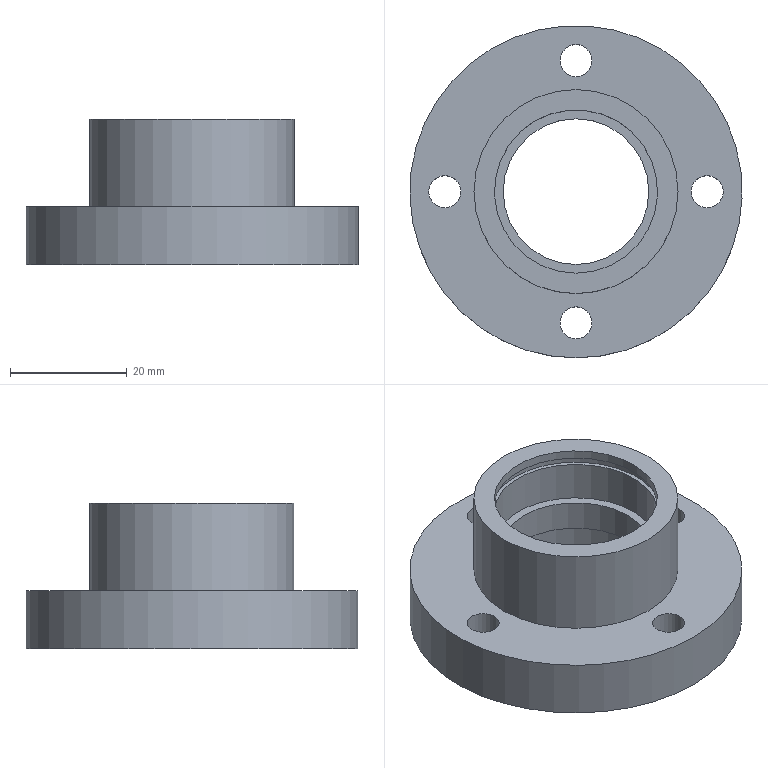Part | NX | features Housing_5003_005_BGRB6902ZZ-25 2 | 1 solid | 30 faces | box 57 x 57 x 25 mm | volume 23135 mm3 | cylinder 17 | plane 13 | commonest cylinder face diameters 5.5 x4 9.5 x4 28 x4 29.4 x2 25 x1 35 x1
STEP:
#1=CARTESIAN_POINT('',(158.525,-336.7,-236.5));
#2=VERTEX_POINT('',#1);
#3=CARTESIAN_POINT('',(158.525,-322.,-236.5));
#4=DIRECTION('',(0.,0.,-1.));
#5=DIRECTION('',(0.,-1.,0.));
#6=AXIS2_PLACEMENT_3D('',#3,#4,#5);
#7=CIRCLE('',#6,14.7);
#8=EDGE_CURVE('',#2,#2,#7,.T.);
#9=ORIENTED_EDGE('',*,*,#8,.T.);
#10=EDGE_LOOP('',(#9));
#11=FACE_BOUND('',#10,.T.);
#12=CARTESIAN_POINT('',(158.525,-336.,-236.5));
#13=VERTEX_POINT('',#12);
#14=CARTESIAN_POINT('',(158.525,-322.,-236.5));
#15=DIRECTION('',(0.,0.,-1.));
#16=DIRECTION('',(0.,-1.,0.));
#17=AXIS2_PLACEMENT_3D('',#14,#15,#16);
#18=CIRCLE('',#17,14.);
#19=EDGE_CURVE('',#13,#13,#18,.T.);
#20=ORIENTED_EDGE('',*,*,#19,.F.);
#21=EDGE_LOOP('',(#20));
#22=FACE_BOUND('',#21,.T.);
#23=CARTESIAN_POINT('',(144.525,-322.,-236.5));
#24=DIRECTION('',(0.,0.,-1.));
#25=DIRECTION('',(0.,-1.,0.));
#26=AXIS2_PLACEMENT_3D('',#23,#24,#25);
#27=PLANE('',#26);
#28=ADVANCED_FACE('',(#11,#22),#27,.T.);
#29=ORIENTED_EDGE('',*,*,#19,.T.);
#30=EDGE_LOOP('',(#29));
#31=FACE_BOUND('',#30,.T.);
#32=CARTESIAN_POINT('',(158.525,-336.,-235.));
#33=VERTEX_POINT('',#32);
#34=CARTESIAN_POINT('',(158.525,-322.,-235.));
#35=DIRECTION('',(0.,0.,-1.));
#36=DIRECTION('',(0.,-1.,0.));
#37=AXIS2_PLACEMENT_3D('',#34,#35,#36);
#38=CIRCLE('',#37,14.);
#39=EDGE_CURVE('',#33,#33,#38,.T.);
#40=ORIENTED_EDGE('',*,*,#39,.F.);
#41=EDGE_LOOP('',(#40));
#42=FACE_BOUND('',#41,.T.);
#43=CARTESIAN_POINT('',(158.525,-322.,-260.));
#44=DIRECTION('',(0.,0.,-1.));
#45=DIRECTION('',(0.,-1.,0.));
#46=AXIS2_PLACEMENT_3D('',#43,#44,#45);
#47=CYLINDRICAL_SURFACE('',#46,14.);
#48=ADVANCED_FACE('',(#31,#42),#47,.F.);
#49=ORIENTED_EDGE('',*,*,#39,.T.);
#50=EDGE_LOOP('',(#49));
#51=FACE_BOUND('',#50,.T.);
#52=CARTESIAN_POINT('',(158.525,-339.5,-235.));
#53=VERTEX_POINT('',#52);
#54=CARTESIAN_POINT('',(158.525,-322.,-235.));
#55=DIRECTION('',(0.,0.,-1.));
#56=DIRECTION('',(0.,-1.,0.));
#57=AXIS2_PLACEMENT_3D('',#54,#55,#56);
#58=CIRCLE('',#57,17.5);
#59=EDGE_CURVE('',#53,#53,#58,.T.);
#60=ORIENTED_EDGE('',*,*,#59,.F.);
#61=EDGE_LOOP('',(#60));
#62=FACE_BOUND('',#61,.T.);
#63=CARTESIAN_POINT('',(141.025,-322.,-235.));
#64=DIRECTION('',(0.,0.,1.));
#65=DIRECTION('',(0.,1.,0.));
#66=AXIS2_PLACEMENT_3D('',#63,#64,#65);
#67=PLANE('',#66);
#68=ADVANCED_FACE('',(#51,#62),#67,.T.);
#69=ORIENTED_EDGE('',*,*,#59,.T.);
#70=EDGE_LOOP('',(#69));
#71=FACE_BOUND('',#70,.T.);
#72=CARTESIAN_POINT('',(158.525,-339.5,-250.));
#73=VERTEX_POINT('',#72);
#74=CARTESIAN_POINT('',(158.525,-322.,-250.));
#75=DIRECTION('',(0.,0.,-1.));
#76=DIRECTION('',(0.,-1.,0.));
#77=AXIS2_PLACEMENT_3D('',#74,#75,#76);
#78=CIRCLE('',#77,17.5);
#79=EDGE_CURVE('',#73,#73,#78,.T.);
#80=ORIENTED_EDGE('',*,*,#79,.F.);
#81=EDGE_LOOP('',(#80));
#82=FACE_BOUND('',#81,.T.);
#83=CARTESIAN_POINT('',(158.525,-322.,-260.));
#84=DIRECTION('',(0.,0.,-1.));
#85=DIRECTION('',(0.,-1.,0.));
#86=AXIS2_PLACEMENT_3D('',#83,#84,#85);
#87=CYLINDRICAL_SURFACE('',#86,17.5);
#88=ADVANCED_FACE('',(#71,#82),#87,.T.);
#89=CARTESIAN_POINT('',(136.025,-319.25,-250.));
#90=VERTEX_POINT('',#89);
#91=CARTESIAN_POINT('',(136.025,-322.,-250.));
#92=DIRECTION('',(0.,0.,1.));
#93=DIRECTION('',(0.,1.,0.));
#94=AXIS2_PLACEMENT_3D('',#91,#92,#93);
#95=CIRCLE('',#94,2.75);
#96=EDGE_CURVE('',#90,#90,#95,.T.);
#97=ORIENTED_EDGE('',*,*,#96,.F.);
#98=EDGE_LOOP('',(#97));
#99=FACE_BOUND('',#98,.T.);
#100=CARTESIAN_POINT('',(158.525,-341.75,-250.));
#101=VERTEX_POINT('',#100);
#102=CARTESIAN_POINT('',(158.525,-344.5,-250.));
#103=DIRECTION('',(0.,0.,1.));
#104=DIRECTION('',(0.,1.,0.));
#105=AXIS2_PLACEMENT_3D('',#102,#103,#104);
#106=CIRCLE('',#105,2.75);
#107=EDGE_CURVE('',#101,#101,#106,.T.);
#108=ORIENTED_EDGE('',*,*,#107,.F.);
#109=EDGE_LOOP('',(#108));
#110=FACE_BOUND('',#109,.T.);
#111=CARTESIAN_POINT('',(158.525,-296.75,-250.));
#112=VERTEX_POINT('',#111);
#113=CARTESIAN_POINT('',(158.525,-299.5,-250.));
#114=DIRECTION('',(0.,0.,1.));
#115=DIRECTION('',(0.,1.,0.));
#116=AXIS2_PLACEMENT_3D('',#113,#114,#115);
#117=CIRCLE('',#116,2.75);
#118=EDGE_CURVE('',#112,#112,#117,.T.);
#119=ORIENTED_EDGE('',*,*,#118,.F.);
#120=EDGE_LOOP('',(#119));
#121=FACE_BOUND('',#120,.T.);
#122=CARTESIAN_POINT('',(181.025,-319.25,-250.));
#123=VERTEX_POINT('',#122);
#124=CARTESIAN_POINT('',(181.025,-322.,-250.));
#125=DIRECTION('',(0.,0.,1.));
#126=DIRECTION('',(0.,1.,0.));
#127=AXIS2_PLACEMENT_3D('',#124,#125,#126);
#128=CIRCLE('',#127,2.75);
#129=EDGE_CURVE('',#123,#123,#128,.T.);
#130=ORIENTED_EDGE('',*,*,#129,.F.);
#131=EDGE_LOOP('',(#130));
#132=FACE_BOUND('',#131,.T.);
#133=ORIENTED_EDGE('',*,*,#79,.T.);
#134=EDGE_LOOP('',(#133));
#135=FACE_BOUND('',#134,.T.);
#136=CARTESIAN_POINT('',(158.525,-350.5,-250.));
#137=VERTEX_POINT('',#136);
#138=CARTESIAN_POINT('',(158.525,-322.,-250.));
#139=DIRECTION('',(0.,0.,-1.));
#140=DIRECTION('',(0.,-1.,0.));
#141=AXIS2_PLACEMENT_3D('',#138,#139,#140);
#142=CIRCLE('',#141,28.5);
#143=EDGE_CURVE('',#137,#137,#142,.T.);
#144=ORIENTED_EDGE('',*,*,#143,.F.);
#145=EDGE_LOOP('',(#144));
#146=FACE_BOUND('',#145,.T.);
#147=CARTESIAN_POINT('',(130.025,-322.,-250.));
#148=DIRECTION('',(0.,0.,1.));
#149=DIRECTION('',(0.,1.,0.));
#150=AXIS2_PLACEMENT_3D('',#147,#148,#149);
#151=PLANE('',#150);
#152=ADVANCED_FACE('',(#99,#110,#121,#132,#135,#146),#151,.T.);
#153=ORIENTED_EDGE('',*,*,#143,.T.);
#154=EDGE_LOOP('',(#153));
#155=FACE_BOUND('',#154,.T.);
#156=CARTESIAN_POINT('',(158.525,-350.5,-260.));
#157=VERTEX_POINT('',#156);
#158=CARTESIAN_POINT('',(158.525,-322.,-260.));
#159=DIRECTION('',(0.,0.,-1.));
#160=DIRECTION('',(0.,-1.,0.));
#161=AXIS2_PLACEMENT_3D('',#158,#159,#160);
#162=CIRCLE('',#161,28.5);
#163=EDGE_CURVE('',#157,#157,#162,.T.);
#164=ORIENTED_EDGE('',*,*,#163,.F.);
#165=EDGE_LOOP('',(#164));
#166=FACE_BOUND('',#165,.T.);
#167=CARTESIAN_POINT('',(158.525,-322.,-260.));
#168=DIRECTION('',(0.,0.,-1.));
#169=DIRECTION('',(0.,-1.,0.));
#170=AXIS2_PLACEMENT_3D('',#167,#168,#169);
#171=CYLINDRICAL_SURFACE('',#170,28.5);
#172=ADVANCED_FACE('',(#155,#166),#171,.T.);
#173=CARTESIAN_POINT('',(136.025,-326.75,-260.));
#174=VERTEX_POINT('',#173);
#175=CARTESIAN_POINT('',(136.025,-322.,-260.));
#176=DIRECTION('',(0.,0.,-1.));
#177=DIRECTION('',(0.,-1.,0.));
#178=AXIS2_PLACEMENT_3D('',#175,#176,#177);
#179=CIRCLE('',#178,4.75);
#180=EDGE_CURVE('',#174,#174,#179,.T.);
#181=ORIENTED_EDGE('',*,*,#180,.F.);
#182=EDGE_LOOP('',(#181));
#183=FACE_BOUND('',#182,.T.);
#184=CARTESIAN_POINT('',(158.525,-349.25,-260.));
#185=VERTEX_POINT('',#184);
#186=CARTESIAN_POINT('',(158.525,-344.5,-260.));
#187=DIRECTION('',(0.,0.,-1.));
#188=DIRECTION('',(0.,-1.,0.));
#189=AXIS2_PLACEMENT_3D('',#186,#187,#188);
#190=CIRCLE('',#189,4.75);
#191=EDGE_CURVE('',#185,#185,#190,.T.);
#192=ORIENTED_EDGE('',*,*,#191,.F.);
#193=EDGE_LOOP('',(#192));
#194=FACE_BOUND('',#193,.T.);
#195=CARTESIAN_POINT('',(158.525,-304.25,-260.));
#196=VERTEX_POINT('',#195);
#197=CARTESIAN_POINT('',(158.525,-299.5,-260.));
#198=DIRECTION('',(0.,0.,-1.));
#199=DIRECTION('',(0.,-1.,0.));
#200=AXIS2_PLACEMENT_3D('',#197,#198,#199);
#201=CIRCLE('',#200,4.75);
#202=EDGE_CURVE('',#196,#196,#201,.T.);
#203=ORIENTED_EDGE('',*,*,#202,.F.);
#204=EDGE_LOOP('',(#203));
#205=FACE_BOUND('',#204,.T.);
#206=CARTESIAN_POINT('',(181.025,-326.75,-260.));
#207=VERTEX_POINT('',#206);
#208=CARTESIAN_POINT('',(181.025,-322.,-260.));
#209=DIRECTION('',(0.,0.,-1.));
#210=DIRECTION('',(0.,-1.,0.));
#211=AXIS2_PLACEMENT_3D('',#208,#209,#210);
#212=CIRCLE('',#211,4.75);
#213=EDGE_CURVE('',#207,#207,#212,.T.);
#214=ORIENTED_EDGE('',*,*,#213,.F.);
#215=EDGE_LOOP('',(#214));
#216=FACE_BOUND('',#215,.T.);
#217=ORIENTED_EDGE('',*,*,#163,.T.);
#218=EDGE_LOOP('',(#217));
#219=FACE_BOUND('',#218,.T.);
#220=CARTESIAN_POINT('',(158.525,-336.,-260.));
#221=VERTEX_POINT('',#220);
#222=CARTESIAN_POINT('',(158.525,-322.,-260.));
#223=DIRECTION('',(0.,0.,-1.));
#224=DIRECTION('',(0.,-1.,0.));
#225=AXIS2_PLACEMENT_3D('',#222,#223,#224);
#226=CIRCLE('',#225,14.);
#227=EDGE_CURVE('',#221,#221,#226,.T.);
#228=ORIENTED_EDGE('',*,*,#227,.F.);
#229=EDGE_LOOP('',(#228));
#230=FACE_BOUND('',#229,.T.);
#231=CARTESIAN_POINT('',(144.525,-322.,-260.));
#232=DIRECTION('',(0.,0.,-1.));
#233=DIRECTION('',(0.,-1.,0.));
#234=AXIS2_PLACEMENT_3D('',#231,#232,#233);
#235=PLANE('',#234);
#236=ADVANCED_FACE('',(#183,#194,#205,#216,#219,#230),#235,.T.);
#237=ORIENTED_EDGE('',*,*,#227,.T.);
#238=EDGE_LOOP('',(#237));
#239=FACE_BOUND('',#238,.T.);
#240=CARTESIAN_POINT('',(158.525,-336.,-258.5));
#241=VERTEX_POINT('',#240);
#242=CARTESIAN_POINT('',(158.525,-322.,-258.5));
#243=DIRECTION('',(0.,0.,-1.));
#244=DIRECTION('',(0.,-1.,0.));
#245=AXIS2_PLACEMENT_3D('',#242,#243,#244);
#246=CIRCLE('',#245,14.);
#247=EDGE_CURVE('',#241,#241,#246,.T.);
#248=ORIENTED_EDGE('',*,*,#247,.F.);
#249=EDGE_LOOP('',(#248));
#250=FACE_BOUND('',#249,.T.);
#251=CARTESIAN_POINT('',(158.525,-322.,-260.));
#252=DIRECTION('',(0.,0.,-1.));
#253=DIRECTION('',(0.,-1.,0.));
#254=AXIS2_PLACEMENT_3D('',#251,#252,#253);
#255=CYLINDRICAL_SURFACE('',#254,14.);
#256=ADVANCED_FACE('',(#239,#250),#255,.F.);
#257=ORIENTED_EDGE('',*,*,#247,.T.);
#258=EDGE_LOOP('',(#257));
#259=FACE_BOUND('',#258,.T.);
#260=CARTESIAN_POINT('',(158.525,-336.7,-258.5));
#261=VERTEX_POINT('',#260);
#262=CARTESIAN_POINT('',(158.525,-322.,-258.5));
#263=DIRECTION('',(0.,0.,-1.));
#264=DIRECTION('',(0.,-1.,0.));
#265=AXIS2_PLACEMENT_3D('',#262,#263,#264);
#266=CIRCLE('',#265,14.7);
#267=EDGE_CURVE('',#261,#261,#266,.T.);
#268=ORIENTED_EDGE('',*,*,#267,.F.);
#269=EDGE_LOOP('',(#268));
#270=FACE_BOUND('',#269,.T.);
#271=CARTESIAN_POINT('',(143.825,-322.,-258.5));
#272=DIRECTION('',(0.,0.,1.));
#273=DIRECTION('',(0.,1.,0.));
#274=AXIS2_PLACEMENT_3D('',#271,#272,#273);
#275=PLANE('',#274);
#276=ADVANCED_FACE('',(#259,#270),#275,.T.);
#277=ORIENTED_EDGE('',*,*,#267,.T.);
#278=EDGE_LOOP('',(#277));
#279=FACE_BOUND('',#278,.T.);
#280=CARTESIAN_POINT('',(158.525,-336.7,-257.15));
#281=VERTEX_POINT('',#280);
#282=CARTESIAN_POINT('',(158.525,-322.,-257.15));
#283=DIRECTION('',(0.,0.,-1.));
#284=DIRECTION('',(0.,-1.,0.));
#285=AXIS2_PLACEMENT_3D('',#282,#283,#284);
#286=CIRCLE('',#285,14.7);
#287=EDGE_CURVE('',#281,#281,#286,.T.);
#288=ORIENTED_EDGE('',*,*,#287,.F.);
#289=EDGE_LOOP('',(#288));
#290=FACE_BOUND('',#289,.T.);
#291=CARTESIAN_POINT('',(158.525,-322.,-260.));
#292=DIRECTION('',(0.,0.,-1.));
#293=DIRECTION('',(0.,-1.,0.));
#294=AXIS2_PLACEMENT_3D('',#291,#292,#293);
#295=CYLINDRICAL_SURFACE('',#294,14.7);
#296=ADVANCED_FACE('',(#279,#290),#295,.F.);
#297=ORIENTED_EDGE('',*,*,#287,.T.);
#298=EDGE_LOOP('',(#297));
#299=FACE_BOUND('',#298,.T.);
#300=CARTESIAN_POINT('',(158.525,-336.,-257.15));
#301=VERTEX_POINT('',#300);
#302=CARTESIAN_POINT('',(158.525,-322.,-257.15));
#303=DIRECTION('',(0.,0.,-1.));
#304=DIRECTION('',(0.,-1.,0.));
#305=AXIS2_PLACEMENT_3D('',#302,#303,#304);
#306=CIRCLE('',#305,14.);
#307=EDGE_CURVE('',#301,#301,#306,.T.);
#308=ORIENTED_EDGE('',*,*,#307,.F.);
#309=EDGE_LOOP('',(#308));
#310=FACE_BOUND('',#309,.T.);
#311=CARTESIAN_POINT('',(144.525,-322.,-257.15));
#312=DIRECTION('',(0.,0.,-1.));
#313=DIRECTION('',(0.,-1.,0.));
#314=AXIS2_PLACEMENT_3D('',#311,#312,#313);
#315=PLANE('',#314);
#316=ADVANCED_FACE('',(#299,#310),#315,.T.);
#317=ORIENTED_EDGE('',*,*,#307,.T.);
#318=EDGE_LOOP('',(#317));
#319=FACE_BOUND('',#318,.T.);
#320=CARTESIAN_POINT('',(158.525,-336.,-250.15));
#321=VERTEX_POINT('',#320);
#322=CARTESIAN_POINT('',(158.525,-322.,-250.15));
#323=DIRECTION('',(0.,0.,-1.));
#324=DIRECTION('',(0.,-1.,0.));
#325=AXIS2_PLACEMENT_3D('',#322,#323,#324);
#326=CIRCLE('',#325,14.);
#327=EDGE_CURVE('',#321,#321,#326,.T.);
#328=ORIENTED_EDGE('',*,*,#327,.F.);
#329=EDGE_LOOP('',(#328));
#330=FACE_BOUND('',#329,.T.);
#331=CARTESIAN_POINT('',(158.525,-322.,-260.));
#332=DIRECTION('',(0.,0.,-1.));
#333=DIRECTION('',(0.,-1.,0.));
#334=AXIS2_PLACEMENT_3D('',#331,#332,#333);
#335=CYLINDRICAL_SURFACE('',#334,14.);
#336=ADVANCED_FACE('',(#319,#330),#335,.F.);
#337=ORIENTED_EDGE('',*,*,#327,.T.);
#338=EDGE_LOOP('',(#337));
#339=FACE_BOUND('',#338,.T.);
#340=CARTESIAN_POINT('',(158.525,-334.5,-250.15));
#341=VERTEX_POINT('',#340);
#342=CARTESIAN_POINT('',(158.525,-322.,-250.15));
#343=DIRECTION('',(0.,0.,-1.));
#344=DIRECTION('',(0.,-1.,0.));
#345=AXIS2_PLACEMENT_3D('',#342,#343,#344);
#346=CIRCLE('',#345,12.5);
#347=EDGE_CURVE('',#341,#341,#346,.T.);
#348=ORIENTED_EDGE('',*,*,#347,.F.);
#349=EDGE_LOOP('',(#348));
#350=FACE_BOUND('',#349,.T.);
#351=CARTESIAN_POINT('',(146.025,-322.,-250.15));
#352=DIRECTION('',(0.,0.,-1.));
#353=DIRECTION('',(0.,-1.,0.));
#354=AXIS2_PLACEMENT_3D('',#351,#352,#353);
#355=PLANE('',#354);
#356=ADVANCED_FACE('',(#339,#350),#355,.T.);
#357=ORIENTED_EDGE('',*,*,#347,.T.);
#358=EDGE_LOOP('',(#357));
#359=FACE_BOUND('',#358,.T.);
#360=CARTESIAN_POINT('',(158.525,-334.5,-244.85));
#361=VERTEX_POINT('',#360);
#362=CARTESIAN_POINT('',(158.525,-322.,-244.85));
#363=DIRECTION('',(0.,0.,-1.));
#364=DIRECTION('',(0.,-1.,0.));
#365=AXIS2_PLACEMENT_3D('',#362,#363,#364);
#366=CIRCLE('',#365,12.5);
#367=EDGE_CURVE('',#361,#361,#366,.T.);
#368=ORIENTED_EDGE('',*,*,#367,.F.);
#369=EDGE_LOOP('',(#368));
#370=FACE_BOUND('',#369,.T.);
#371=CARTESIAN_POINT('',(158.525,-322.,-260.));
#372=DIRECTION('',(0.,0.,-1.));
#373=DIRECTION('',(0.,-1.,0.));
#374=AXIS2_PLACEMENT_3D('',#371,#372,#373);
#375=CYLINDRICAL_SURFACE('',#374,12.5);
#376=ADVANCED_FACE('',(#359,#370),#375,.F.);
#377=ORIENTED_EDGE('',*,*,#367,.T.);
#378=EDGE_LOOP('',(#377));
#379=FACE_BOUND('',#378,.T.);
#380=CARTESIAN_POINT('',(158.525,-336.,-244.85));
#381=VERTEX_POINT('',#380);
#382=CARTESIAN_POINT('',(158.525,-322.,-244.85));
#383=DIRECTION('',(0.,0.,-1.));
#384=DIRECTION('',(0.,-1.,0.));
#385=AXIS2_PLACEMENT_3D('',#382,#383,#384);
#386=CIRCLE('',#385,14.);
#387=EDGE_CURVE('',#381,#381,#386,.T.);
#388=ORIENTED_EDGE('',*,*,#387,.F.);
#389=EDGE_LOOP('',(#388));
#390=FACE_BOUND('',#389,.T.);
#391=CARTESIAN_POINT('',(144.525,-322.,-244.85));
#392=DIRECTION('',(0.,0.,1.));
#393=DIRECTION('',(0.,1.,0.));
#394=AXIS2_PLACEMENT_3D('',#391,#392,#393);
#395=PLANE('',#394);
#396=ADVANCED_FACE('',(#379,#390),#395,.T.);
#397=ORIENTED_EDGE('',*,*,#387,.T.);
#398=EDGE_LOOP('',(#397));
#399=FACE_BOUND('',#398,.T.);
#400=CARTESIAN_POINT('',(158.525,-336.,-237.85));
#401=VERTEX_POINT('',#400);
#402=CARTESIAN_POINT('',(158.525,-322.,-237.85));
#403=DIRECTION('',(0.,0.,-1.));
#404=DIRECTION('',(0.,-1.,0.));
#405=AXIS2_PLACEMENT_3D('',#402,#403,#404);
#406=CIRCLE('',#405,14.);
#407=EDGE_CURVE('',#401,#401,#406,.T.);
#408=ORIENTED_EDGE('',*,*,#407,.F.);
#409=EDGE_LOOP('',(#408));
#410=FACE_BOUND('',#409,.T.);
#411=CARTESIAN_POINT('',(158.525,-322.,-260.));
#412=DIRECTION('',(0.,0.,-1.));
#413=DIRECTION('',(0.,-1.,0.));
#414=AXIS2_PLACEMENT_3D('',#411,#412,#413);
#415=CYLINDRICAL_SURFACE('',#414,14.);
#416=ADVANCED_FACE('',(#399,#410),#415,.F.);
#417=ORIENTED_EDGE('',*,*,#407,.T.);
#418=EDGE_LOOP('',(#417));
#419=FACE_BOUND('',#418,.T.);
#420=CARTESIAN_POINT('',(158.525,-336.7,-237.85));
#421=VERTEX_POINT('',#420);
#422=CARTESIAN_POINT('',(158.525,-322.,-237.85));
#423=DIRECTION('',(0.,0.,-1.));
#424=DIRECTION('',(0.,-1.,0.));
#425=AXIS2_PLACEMENT_3D('',#422,#423,#424);
#426=CIRCLE('',#425,14.7);
#427=EDGE_CURVE('',#421,#421,#426,.T.);
#428=ORIENTED_EDGE('',*,*,#427,.F.);
#429=EDGE_LOOP('',(#428));
#430=FACE_BOUND('',#429,.T.);
#431=CARTESIAN_POINT('',(143.825,-322.,-237.85));
#432=DIRECTION('',(0.,0.,1.));
#433=DIRECTION('',(0.,1.,0.));
#434=AXIS2_PLACEMENT_3D('',#431,#432,#433);
#435=PLANE('',#434);
#436=ADVANCED_FACE('',(#419,#430),#435,.T.);
#437=ORIENTED_EDGE('',*,*,#427,.T.);
#438=EDGE_LOOP('',(#437));
#439=FACE_BOUND('',#438,.T.);
#440=ORIENTED_EDGE('',*,*,#8,.F.);
#441=EDGE_LOOP('',(#440));
#442=FACE_BOUND('',#441,.T.);
#443=CARTESIAN_POINT('',(158.525,-322.,-260.));
#444=DIRECTION('',(0.,0.,-1.));
#445=DIRECTION('',(0.,-1.,0.));
#446=AXIS2_PLACEMENT_3D('',#443,#444,#445);
#447=CYLINDRICAL_SURFACE('',#446,14.7);
#448=ADVANCED_FACE('',(#439,#442),#447,.F.);
#449=ORIENTED_EDGE('',*,*,#129,.T.);
#450=EDGE_LOOP('',(#449));
#451=FACE_BOUND('',#450,.T.);
#452=CARTESIAN_POINT('',(181.025,-324.75,-254.9));
#453=VERTEX_POINT('',#452);
#454=CARTESIAN_POINT('',(181.025,-322.,-254.9));
#455=DIRECTION('',(0.,0.,-1.));
#456=DIRECTION('',(0.,-1.,0.));
#457=AXIS2_PLACEMENT_3D('',#454,#455,#456);
#458=CIRCLE('',#457,2.75);
#459=EDGE_CURVE('',#453,#453,#458,.T.);
#460=ORIENTED_EDGE('',*,*,#459,.T.);
#461=EDGE_LOOP('',(#460));
#462=FACE_BOUND('',#461,.T.);
#463=CARTESIAN_POINT('',(181.025,-322.,-260.));
#464=DIRECTION('',(0.,0.,-1.));
#465=DIRECTION('',(0.,-1.,0.));
#466=AXIS2_PLACEMENT_3D('',#463,#464,#465);
#467=CYLINDRICAL_SURFACE('',#466,2.75);
#468=ADVANCED_FACE('',(#451,#462),#467,.F.);
#469=ORIENTED_EDGE('',*,*,#459,.F.);
#470=EDGE_LOOP('',(#469));
#471=FACE_BOUND('',#470,.T.);
#472=CARTESIAN_POINT('',(181.025,-326.75,-254.9));
#473=VERTEX_POINT('',#472);
#474=CARTESIAN_POINT('',(181.025,-322.,-254.9));
#475=DIRECTION('',(0.,0.,-1.));
#476=DIRECTION('',(0.,-1.,0.));
#477=AXIS2_PLACEMENT_3D('',#474,#475,#476);
#478=CIRCLE('',#477,4.75);
#479=EDGE_CURVE('',#473,#473,#478,.T.);
#480=ORIENTED_EDGE('',*,*,#479,.T.);
#481=EDGE_LOOP('',(#480));
#482=FACE_BOUND('',#481,.T.);
#483=CARTESIAN_POINT('',(178.275,-322.,-254.9));
#484=DIRECTION('',(0.,0.,1.));
#485=DIRECTION('',(0.,1.,0.));
#486=AXIS2_PLACEMENT_3D('',#483,#484,#485);
#487=PLANE('',#486);
#488=ADVANCED_FACE('',(#471,#482),#487,.F.);
#489=ORIENTED_EDGE('',*,*,#479,.F.);
#490=EDGE_LOOP('',(#489));
#491=FACE_BOUND('',#490,.T.);
#492=ORIENTED_EDGE('',*,*,#213,.T.);
#493=EDGE_LOOP('',(#492));
#494=FACE_BOUND('',#493,.T.);
#495=CARTESIAN_POINT('',(181.025,-322.,-260.));
#496=DIRECTION('',(0.,0.,-1.));
#497=DIRECTION('',(0.,-1.,0.));
#498=AXIS2_PLACEMENT_3D('',#495,#496,#497);
#499=CYLINDRICAL_SURFACE('',#498,4.75);
#500=ADVANCED_FACE('',(#491,#494),#499,.F.);
#501=ORIENTED_EDGE('',*,*,#118,.T.);
#502=EDGE_LOOP('',(#501));
#503=FACE_BOUND('',#502,.T.);
#504=CARTESIAN_POINT('',(158.525,-302.25,-254.9));
#505=VERTEX_POINT('',#504);
#506=CARTESIAN_POINT('',(158.525,-299.5,-254.9));
#507=DIRECTION('',(0.,0.,-1.));
#508=DIRECTION('',(0.,-1.,0.));
#509=AXIS2_PLACEMENT_3D('',#506,#507,#508);
#510=CIRCLE('',#509,2.75);
#511=EDGE_CURVE('',#505,#505,#510,.T.);
#512=ORIENTED_EDGE('',*,*,#511,.T.);
#513=EDGE_LOOP('',(#512));
#514=FACE_BOUND('',#513,.T.);
#515=CARTESIAN_POINT('',(158.525,-299.5,-260.));
#516=DIRECTION('',(0.,0.,-1.));
#517=DIRECTION('',(0.,-1.,0.));
#518=AXIS2_PLACEMENT_3D('',#515,#516,#517);
#519=CYLINDRICAL_SURFACE('',#518,2.75);
#520=ADVANCED_FACE('',(#503,#514),#519,.F.);
#521=ORIENTED_EDGE('',*,*,#511,.F.);
#522=EDGE_LOOP('',(#521));
#523=FACE_BOUND('',#522,.T.);
#524=CARTESIAN_POINT('',(158.525,-304.25,-254.9));
#525=VERTEX_POINT('',#524);
#526=CARTESIAN_POINT('',(158.525,-299.5,-254.9));
#527=DIRECTION('',(0.,0.,-1.));
#528=DIRECTION('',(0.,-1.,0.));
#529=AXIS2_PLACEMENT_3D('',#526,#527,#528);
#530=CIRCLE('',#529,4.75);
#531=EDGE_CURVE('',#525,#525,#530,.T.);
#532=ORIENTED_EDGE('',*,*,#531,.T.);
#533=EDGE_LOOP('',(#532));
#534=FACE_BOUND('',#533,.T.);
#535=CARTESIAN_POINT('',(155.775,-299.5,-254.9));
#536=DIRECTION('',(0.,0.,1.));
#537=DIRECTION('',(0.,1.,0.));
#538=AXIS2_PLACEMENT_3D('',#535,#536,#537);
#539=PLANE('',#538);
#540=ADVANCED_FACE('',(#523,#534),#539,.F.);
#541=ORIENTED_EDGE('',*,*,#531,.F.);
#542=EDGE_LOOP('',(#541));
#543=FACE_BOUND('',#542,.T.);
#544=ORIENTED_EDGE('',*,*,#202,.T.);
#545=EDGE_LOOP('',(#544));
#546=FACE_BOUND('',#545,.T.);
#547=CARTESIAN_POINT('',(158.525,-299.5,-260.));
#548=DIRECTION('',(0.,0.,-1.));
#549=DIRECTION('',(0.,-1.,0.));
#550=AXIS2_PLACEMENT_3D('',#547,#548,#549);
#551=CYLINDRICAL_SURFACE('',#550,4.75);
#552=ADVANCED_FACE('',(#543,#546),#551,.F.);
#553=ORIENTED_EDGE('',*,*,#107,.T.);
#554=EDGE_LOOP('',(#553));
#555=FACE_BOUND('',#554,.T.);
#556=CARTESIAN_POINT('',(158.525,-347.25,-254.9));
#557=VERTEX_POINT('',#556);
#558=CARTESIAN_POINT('',(158.525,-344.5,-254.9));
#559=DIRECTION('',(0.,0.,-1.));
#560=DIRECTION('',(0.,-1.,0.));
#561=AXIS2_PLACEMENT_3D('',#558,#559,#560);
#562=CIRCLE('',#561,2.75);
#563=EDGE_CURVE('',#557,#557,#562,.T.);
#564=ORIENTED_EDGE('',*,*,#563,.T.);
#565=EDGE_LOOP('',(#564));
#566=FACE_BOUND('',#565,.T.);
#567=CARTESIAN_POINT('',(158.525,-344.5,-260.));
#568=DIRECTION('',(0.,0.,-1.));
#569=DIRECTION('',(0.,-1.,0.));
#570=AXIS2_PLACEMENT_3D('',#567,#568,#569);
#571=CYLINDRICAL_SURFACE('',#570,2.75);
#572=ADVANCED_FACE('',(#555,#566),#571,.F.);
#573=ORIENTED_EDGE('',*,*,#563,.F.);
#574=EDGE_LOOP('',(#573));
#575=FACE_BOUND('',#574,.T.);
#576=CARTESIAN_POINT('',(158.525,-349.25,-254.9));
#577=VERTEX_POINT('',#576);
#578=CARTESIAN_POINT('',(158.525,-344.5,-254.9));
#579=DIRECTION('',(0.,0.,-1.));
#580=DIRECTION('',(0.,-1.,0.));
#581=AXIS2_PLACEMENT_3D('',#578,#579,#580);
#582=CIRCLE('',#581,4.75);
#583=EDGE_CURVE('',#577,#577,#582,.T.);
#584=ORIENTED_EDGE('',*,*,#583,.T.);
#585=EDGE_LOOP('',(#584));
#586=FACE_BOUND('',#585,.T.);
#587=CARTESIAN_POINT('',(155.775,-344.5,-254.9));
#588=DIRECTION('',(0.,0.,1.));
#589=DIRECTION('',(0.,1.,0.));
#590=AXIS2_PLACEMENT_3D('',#587,#588,#589);
#591=PLANE('',#590);
#592=ADVANCED_FACE('',(#575,#586),#591,.F.);
#593=ORIENTED_EDGE('',*,*,#583,.F.);
#594=EDGE_LOOP('',(#593));
#595=FACE_BOUND('',#594,.T.);
#596=ORIENTED_EDGE('',*,*,#191,.T.);
#597=EDGE_LOOP('',(#596));
#598=FACE_BOUND('',#597,.T.);
#599=CARTESIAN_POINT('',(158.525,-344.5,-260.));
#600=DIRECTION('',(0.,0.,-1.));
#601=DIRECTION('',(0.,-1.,0.));
#602=AXIS2_PLACEMENT_3D('',#599,#600,#601);
#603=CYLINDRICAL_SURFACE('',#602,4.75);
#604=ADVANCED_FACE('',(#595,#598),#603,.F.);
#605=ORIENTED_EDGE('',*,*,#96,.T.);
#606=EDGE_LOOP('',(#605));
#607=FACE_BOUND('',#606,.T.);
#608=CARTESIAN_POINT('',(136.025,-324.75,-254.9));
#609=VERTEX_POINT('',#608);
#610=CARTESIAN_POINT('',(136.025,-322.,-254.9));
#611=DIRECTION('',(0.,0.,-1.));
#612=DIRECTION('',(0.,-1.,0.));
#613=AXIS2_PLACEMENT_3D('',#610,#611,#612);
#614=CIRCLE('',#613,2.75);
#615=EDGE_CURVE('',#609,#609,#614,.T.);
#616=ORIENTED_EDGE('',*,*,#615,.T.);
#617=EDGE_LOOP('',(#616));
#618=FACE_BOUND('',#617,.T.);
#619=CARTESIAN_POINT('',(136.025,-322.,-260.));
#620=DIRECTION('',(0.,0.,-1.));
#621=DIRECTION('',(0.,-1.,0.));
#622=AXIS2_PLACEMENT_3D('',#619,#620,#621);
#623=CYLINDRICAL_SURFACE('',#622,2.75);
#624=ADVANCED_FACE('',(#607,#618),#623,.F.);
#625=ORIENTED_EDGE('',*,*,#615,.F.);
#626=EDGE_LOOP('',(#625));
#627=FACE_BOUND('',#626,.T.);
#628=CARTESIAN_POINT('',(136.025,-326.75,-254.9));
#629=VERTEX_POINT('',#628);
#630=CARTESIAN_POINT('',(136.025,-322.,-254.9));
#631=DIRECTION('',(0.,0.,-1.));
#632=DIRECTION('',(0.,-1.,0.));
#633=AXIS2_PLACEMENT_3D('',#630,#631,#632);
#634=CIRCLE('',#633,4.75);
#635=EDGE_CURVE('',#629,#629,#634,.T.);
#636=ORIENTED_EDGE('',*,*,#635,.T.);
#637=EDGE_LOOP('',(#636));
#638=FACE_BOUND('',#637,.T.);
#639=CARTESIAN_POINT('',(133.275,-322.,-254.9));
#640=DIRECTION('',(0.,0.,1.));
#641=DIRECTION('',(0.,1.,0.));
#642=AXIS2_PLACEMENT_3D('',#639,#640,#641);
#643=PLANE('',#642);
#644=ADVANCED_FACE('',(#627,#638),#643,.F.);
#645=ORIENTED_EDGE('',*,*,#635,.F.);
#646=EDGE_LOOP('',(#645));
#647=FACE_BOUND('',#646,.T.);
#648=ORIENTED_EDGE('',*,*,#180,.T.);
#649=EDGE_LOOP('',(#648));
#650=FACE_BOUND('',#649,.T.);
#651=CARTESIAN_POINT('',(136.025,-322.,-260.));
#652=DIRECTION('',(0.,0.,-1.));
#653=DIRECTION('',(0.,-1.,0.));
#654=AXIS2_PLACEMENT_3D('',#651,#652,#653);
#655=CYLINDRICAL_SURFACE('',#654,4.75);
#656=ADVANCED_FACE('',(#647,#650),#655,.F.);
#657=CLOSED_SHELL('',(#28,#48,#68,#88,#152,#172,#236,#256,#276,#296,#316,#336,#356,#376,#396,#416,#436,#448,#468,#488,#500,#520,#540,#552,#572,#592,#604,#624,#644,#656));
#658=MANIFOLD_SOLID_BREP('',#657);
#659=(LENGTH_UNIT()NAMED_UNIT(*)SI_UNIT(.MILLI.,.METRE.));
#660=UNCERTAINTY_MEASURE_WITH_UNIT(LENGTH_MEASURE(0.00001),#659,'','');
#661=(NAMED_UNIT(*)PLANE_ANGLE_UNIT()SI_UNIT($,.RADIAN.));
#662=(NAMED_UNIT(*)SI_UNIT($,.STERADIAN.)SOLID_ANGLE_UNIT());
#663=(GEOMETRIC_REPRESENTATION_CONTEXT(3)GLOBAL_UNCERTAINTY_ASSIGNED_CONTEXT((#660))GLOBAL_UNIT_ASSIGNED_CONTEXT((#659,#661,#662))REPRESENTATION_CONTEXT('',''));
#664=ADVANCED_BREP_SHAPE_REPRESENTATION('',(#658),#663);